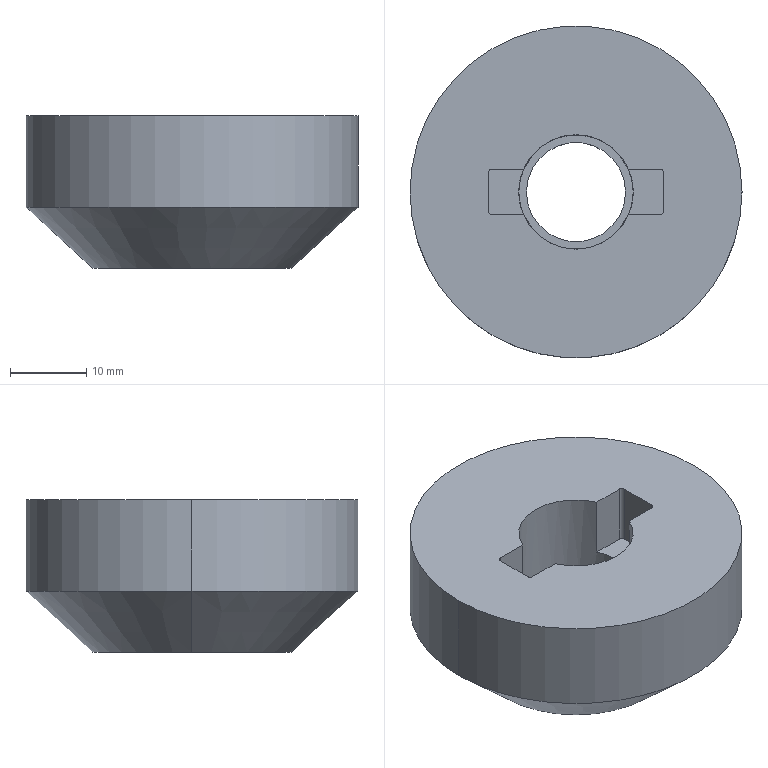Part | SolidWorks | features ICE 2, Blend 1, Extrusion 1 | 1 solid | 23 faces | box 43.5 x 43.5 x 20 mm | volume 21997 mm3 | plane 11 | cylinder 10 | cone 2 | commonest cylinder face diameters 1 x4 13 x2 15 x2 43.5 x2
STEP:
#1=CARTESIAN_POINT('',(6.5,0.,-8.));
#2=VERTEX_POINT('',#1);
#3=CARTESIAN_POINT('',(-6.5,0.,-8.));
#4=VERTEX_POINT('',#3);
#5=CARTESIAN_POINT('',(0.,0.,-8.));
#6=DIRECTION('',(0.,0.,-1.));
#7=DIRECTION('',(-1.,0.,0.));
#8=AXIS2_PLACEMENT_3D('',#5,#6,#7);
#9=CIRCLE('',#8,6.5);
#10=EDGE_CURVE('',#2,#4,#9,.T.);
#11=ORIENTED_EDGE('',*,*,#10,.T.);
#12=CARTESIAN_POINT('',(-6.5,0.,0.));
#13=VERTEX_POINT('',#12);
#14=CARTESIAN_POINT('',(-6.5,0.,-48.));
#15=DIRECTION('',(0.,0.,1.));
#16=VECTOR('',#15,1000.);
#17=LINE('',#14,#16);
#18=EDGE_CURVE('',#4,#13,#17,.T.);
#19=ORIENTED_EDGE('',*,*,#18,.T.);
#20=CARTESIAN_POINT('',(6.5,0.,0.));
#21=VERTEX_POINT('',#20);
#22=CARTESIAN_POINT('',(0.,0.,0.));
#23=DIRECTION('',(0.,0.,1.));
#24=DIRECTION('',(1.,0.,0.));
#25=AXIS2_PLACEMENT_3D('',#22,#23,#24);
#26=CIRCLE('',#25,6.5);
#27=EDGE_CURVE('',#13,#21,#26,.T.);
#28=ORIENTED_EDGE('',*,*,#27,.T.);
#29=CARTESIAN_POINT('',(6.5,0.,-48.));
#30=DIRECTION('',(0.,0.,1.));
#31=VECTOR('',#30,1000.);
#32=LINE('',#29,#31);
#33=EDGE_CURVE('',#2,#21,#32,.T.);
#34=ORIENTED_EDGE('',*,*,#33,.F.);
#35=EDGE_LOOP('',(#11,#19,#28,#34));
#36=FACE_OUTER_BOUND('',#35,.T.);
#37=CARTESIAN_POINT('',(0.,0.,-48.));
#38=DIRECTION('',(0.,0.,1.));
#39=DIRECTION('',(1.,0.,0.));
#40=AXIS2_PLACEMENT_3D('',#37,#38,#39);
#41=CYLINDRICAL_SURFACE('',#40,6.5);
#42=ADVANCED_FACE('',(#36),#41,.F.);
#43=CARTESIAN_POINT('',(-13.,0.,-8.));
#44=VERTEX_POINT('',#43);
#45=CARTESIAN_POINT('',(13.,0.,-8.));
#46=VERTEX_POINT('',#45);
#47=CARTESIAN_POINT('',(0.,0.,-8.));
#48=DIRECTION('',(0.,0.,-1.));
#49=DIRECTION('',(-1.,0.,0.));
#50=AXIS2_PLACEMENT_3D('',#47,#48,#49);
#51=CIRCLE('',#50,13.);
#52=EDGE_CURVE('',#44,#46,#51,.T.);
#53=ORIENTED_EDGE('',*,*,#52,.F.);
#54=CARTESIAN_POINT('',(-21.75,0.,0.));
#55=VERTEX_POINT('',#54);
#56=CARTESIAN_POINT('',(-13.,0.,-8.));
#57=DIRECTION('',(-0.738,0.,0.6748));
#58=VECTOR('',#57,1000.);
#59=LINE('',#56,#58);
#60=EDGE_CURVE('',#44,#55,#59,.T.);
#61=ORIENTED_EDGE('',*,*,#60,.T.);
#62=CARTESIAN_POINT('',(21.75,0.,0.));
#63=VERTEX_POINT('',#62);
#64=CARTESIAN_POINT('',(0.,0.,0.));
#65=DIRECTION('',(0.,0.,-1.));
#66=DIRECTION('',(-1.,0.,0.));
#67=AXIS2_PLACEMENT_3D('',#64,#65,#66);
#68=CIRCLE('',#67,21.75);
#69=EDGE_CURVE('',#55,#63,#68,.T.);
#70=ORIENTED_EDGE('',*,*,#69,.T.);
#71=CARTESIAN_POINT('',(13.,0.,-8.));
#72=DIRECTION('',(0.738,0.,0.6748));
#73=VECTOR('',#72,1000.);
#74=LINE('',#71,#73);
#75=EDGE_CURVE('',#46,#63,#74,.T.);
#76=ORIENTED_EDGE('',*,*,#75,.F.);
#77=EDGE_LOOP('',(#53,#61,#70,#76));
#78=FACE_OUTER_BOUND('',#77,.T.);
#79=CARTESIAN_POINT('',(0.,0.,-8.));
#80=DIRECTION('',(0.,0.,1.));
#81=DIRECTION('',(1.,0.,0.));
#82=AXIS2_PLACEMENT_3D('',#79,#80,#81);
#83=CONICAL_SURFACE('',#82,13.,0.8301);
#84=ADVANCED_FACE('',(#78),#83,.T.);
#85=CARTESIAN_POINT('',(7.5,0.,4.));
#86=VERTEX_POINT('',#85);
#87=CARTESIAN_POINT('',(6.874,-3.,4.));
#88=VERTEX_POINT('',#87);
#89=CARTESIAN_POINT('',(0.,0.,4.));
#90=DIRECTION('',(0.,0.,-1.));
#91=DIRECTION('',(-1.,0.,0.));
#92=AXIS2_PLACEMENT_3D('',#89,#90,#91);
#93=CIRCLE('',#92,7.5);
#94=EDGE_CURVE('',#86,#88,#93,.T.);
#95=ORIENTED_EDGE('',*,*,#94,.F.);
#96=CARTESIAN_POINT('',(7.5,0.,0.));
#97=VERTEX_POINT('',#96);
#98=CARTESIAN_POINT('',(7.5,0.,12.));
#99=DIRECTION('',(0.,0.,-1.));
#100=VECTOR('',#99,1000.);
#101=LINE('',#98,#100);
#102=EDGE_CURVE('',#86,#97,#101,.T.);
#103=ORIENTED_EDGE('',*,*,#102,.T.);
#104=CARTESIAN_POINT('',(-7.5,0.,0.));
#105=VERTEX_POINT('',#104);
#106=CARTESIAN_POINT('',(0.,0.,0.));
#107=DIRECTION('',(0.,0.,1.));
#108=DIRECTION('',(1.,0.,0.));
#109=AXIS2_PLACEMENT_3D('',#106,#107,#108);
#110=CIRCLE('',#109,7.5);
#111=EDGE_CURVE('',#105,#97,#110,.T.);
#112=ORIENTED_EDGE('',*,*,#111,.F.);
#113=CARTESIAN_POINT('',(-7.5,0.,4.));
#114=VERTEX_POINT('',#113);
#115=CARTESIAN_POINT('',(-7.5,0.,12.));
#116=DIRECTION('',(0.,0.,-1.));
#117=VECTOR('',#116,1000.);
#118=LINE('',#115,#117);
#119=EDGE_CURVE('',#114,#105,#118,.T.);
#120=ORIENTED_EDGE('',*,*,#119,.F.);
#121=CARTESIAN_POINT('',(-6.874,-3.,4.));
#122=VERTEX_POINT('',#121);
#123=CARTESIAN_POINT('',(0.,0.,4.));
#124=DIRECTION('',(0.,0.,-1.));
#125=DIRECTION('',(-1.,0.,0.));
#126=AXIS2_PLACEMENT_3D('',#123,#124,#125);
#127=CIRCLE('',#126,7.5);
#128=EDGE_CURVE('',#122,#114,#127,.T.);
#129=ORIENTED_EDGE('',*,*,#128,.F.);
#130=CARTESIAN_POINT('',(-6.874,-3.,12.));
#131=VERTEX_POINT('',#130);
#132=CARTESIAN_POINT('',(-6.874,-3.,12.));
#133=DIRECTION('',(0.,0.,-1.));
#134=VECTOR('',#133,1000.);
#135=LINE('',#132,#134);
#136=EDGE_CURVE('',#131,#122,#135,.T.);
#137=ORIENTED_EDGE('',*,*,#136,.F.);
#138=CARTESIAN_POINT('',(6.874,-3.,12.));
#139=VERTEX_POINT('',#138);
#140=CARTESIAN_POINT('',(0.,0.,12.));
#141=DIRECTION('',(0.,0.,1.));
#142=DIRECTION('',(1.,0.,0.));
#143=AXIS2_PLACEMENT_3D('',#140,#141,#142);
#144=CIRCLE('',#143,7.5);
#145=EDGE_CURVE('',#131,#139,#144,.T.);
#146=ORIENTED_EDGE('',*,*,#145,.T.);
#147=CARTESIAN_POINT('',(6.874,-3.,12.));
#148=DIRECTION('',(0.,0.,1.));
#149=VECTOR('',#148,1000.);
#150=LINE('',#147,#149);
#151=EDGE_CURVE('',#88,#139,#150,.T.);
#152=ORIENTED_EDGE('',*,*,#151,.F.);
#153=EDGE_LOOP('',(#95,#103,#112,#120,#129,#137,#146,#152));
#154=FACE_OUTER_BOUND('',#153,.T.);
#155=CARTESIAN_POINT('',(0.,0.,12.));
#156=DIRECTION('',(0.,0.,-1.));
#157=DIRECTION('',(-1.,0.,0.));
#158=AXIS2_PLACEMENT_3D('',#155,#156,#157);
#159=CYLINDRICAL_SURFACE('',#158,7.5);
#160=ADVANCED_FACE('',(#154),#159,.F.);
#161=CARTESIAN_POINT('',(21.75,0.,12.));
#162=VERTEX_POINT('',#161);
#163=CARTESIAN_POINT('',(-21.75,0.,12.));
#164=VERTEX_POINT('',#163);
#165=CARTESIAN_POINT('',(0.,0.,12.));
#166=DIRECTION('',(0.,0.,1.));
#167=DIRECTION('',(1.,0.,0.));
#168=AXIS2_PLACEMENT_3D('',#165,#166,#167);
#169=CIRCLE('',#168,21.75);
#170=EDGE_CURVE('',#162,#164,#169,.T.);
#171=ORIENTED_EDGE('',*,*,#170,.F.);
#172=CARTESIAN_POINT('',(21.75,0.,12.));
#173=DIRECTION('',(0.,0.,-1.));
#174=VECTOR('',#173,1000.);
#175=LINE('',#172,#174);
#176=EDGE_CURVE('',#162,#63,#175,.T.);
#177=ORIENTED_EDGE('',*,*,#176,.T.);
#178=ORIENTED_EDGE('',*,*,#69,.F.);
#179=CARTESIAN_POINT('',(-21.75,0.,12.));
#180=DIRECTION('',(0.,0.,-1.));
#181=VECTOR('',#180,1000.);
#182=LINE('',#179,#181);
#183=EDGE_CURVE('',#164,#55,#182,.T.);
#184=ORIENTED_EDGE('',*,*,#183,.F.);
#185=EDGE_LOOP('',(#171,#177,#178,#184));
#186=FACE_OUTER_BOUND('',#185,.T.);
#187=CARTESIAN_POINT('',(0.,0.,12.));
#188=DIRECTION('',(0.,0.,-1.));
#189=DIRECTION('',(-1.,0.,0.));
#190=AXIS2_PLACEMENT_3D('',#187,#188,#189);
#191=CYLINDRICAL_SURFACE('',#190,21.75);
#192=ADVANCED_FACE('',(#186),#191,.T.);
#193=CARTESIAN_POINT('',(11.,-3.,12.));
#194=VERTEX_POINT('',#193);
#195=CARTESIAN_POINT('',(-11.,-3.,12.));
#196=DIRECTION('',(1.,0.,0.));
#197=VECTOR('',#196,1000.);
#198=LINE('',#195,#197);
#199=EDGE_CURVE('',#139,#194,#198,.T.);
#200=ORIENTED_EDGE('',*,*,#199,.F.);
#201=ORIENTED_EDGE('',*,*,#145,.F.);
#202=CARTESIAN_POINT('',(-11.,-3.,12.));
#203=VERTEX_POINT('',#202);
#204=CARTESIAN_POINT('',(-11.,-3.,12.));
#205=DIRECTION('',(1.,0.,0.));
#206=VECTOR('',#205,1000.);
#207=LINE('',#204,#206);
#208=EDGE_CURVE('',#203,#131,#207,.T.);
#209=ORIENTED_EDGE('',*,*,#208,.F.);
#210=CARTESIAN_POINT('',(-11.5,-2.5,12.));
#211=VERTEX_POINT('',#210);
#212=CARTESIAN_POINT('',(-11.,-2.5,12.));
#213=DIRECTION('',(0.,0.,1.));
#214=DIRECTION('',(1.,0.,0.));
#215=AXIS2_PLACEMENT_3D('',#212,#213,#214);
#216=CIRCLE('',#215,0.5);
#217=EDGE_CURVE('',#211,#203,#216,.T.);
#218=ORIENTED_EDGE('',*,*,#217,.F.);
#219=CARTESIAN_POINT('',(-11.5,2.5,12.));
#220=VERTEX_POINT('',#219);
#221=CARTESIAN_POINT('',(-11.5,2.5,12.));
#222=DIRECTION('',(0.,-1.,0.));
#223=VECTOR('',#222,1000.);
#224=LINE('',#221,#223);
#225=EDGE_CURVE('',#220,#211,#224,.T.);
#226=ORIENTED_EDGE('',*,*,#225,.F.);
#227=CARTESIAN_POINT('',(-11.,3.,12.));
#228=VERTEX_POINT('',#227);
#229=CARTESIAN_POINT('',(-11.,2.5,12.));
#230=DIRECTION('',(0.,0.,1.));
#231=DIRECTION('',(1.,0.,0.));
#232=AXIS2_PLACEMENT_3D('',#229,#230,#231);
#233=CIRCLE('',#232,0.5);
#234=EDGE_CURVE('',#228,#220,#233,.T.);
#235=ORIENTED_EDGE('',*,*,#234,.F.);
#236=CARTESIAN_POINT('',(-6.874,3.,12.));
#237=VERTEX_POINT('',#236);
#238=CARTESIAN_POINT('',(-11.,3.,12.));
#239=DIRECTION('',(-1.,0.,0.));
#240=VECTOR('',#239,1000.);
#241=LINE('',#238,#240);
#242=EDGE_CURVE('',#237,#228,#241,.T.);
#243=ORIENTED_EDGE('',*,*,#242,.F.);
#244=CARTESIAN_POINT('',(6.874,3.,12.));
#245=VERTEX_POINT('',#244);
#246=CARTESIAN_POINT('',(0.,0.,12.));
#247=DIRECTION('',(0.,0.,1.));
#248=DIRECTION('',(1.,0.,0.));
#249=AXIS2_PLACEMENT_3D('',#246,#247,#248);
#250=CIRCLE('',#249,7.5);
#251=EDGE_CURVE('',#245,#237,#250,.T.);
#252=ORIENTED_EDGE('',*,*,#251,.F.);
#253=CARTESIAN_POINT('',(11.,3.,12.));
#254=VERTEX_POINT('',#253);
#255=CARTESIAN_POINT('',(-11.,3.,12.));
#256=DIRECTION('',(-1.,0.,0.));
#257=VECTOR('',#256,1000.);
#258=LINE('',#255,#257);
#259=EDGE_CURVE('',#254,#245,#258,.T.);
#260=ORIENTED_EDGE('',*,*,#259,.F.);
#261=CARTESIAN_POINT('',(11.5,2.5,12.));
#262=VERTEX_POINT('',#261);
#263=CARTESIAN_POINT('',(11.,2.5,12.));
#264=DIRECTION('',(0.,0.,1.));
#265=DIRECTION('',(-1.,0.,0.));
#266=AXIS2_PLACEMENT_3D('',#263,#264,#265);
#267=CIRCLE('',#266,0.5);
#268=EDGE_CURVE('',#262,#254,#267,.T.);
#269=ORIENTED_EDGE('',*,*,#268,.F.);
#270=CARTESIAN_POINT('',(11.5,-2.5,12.));
#271=VERTEX_POINT('',#270);
#272=CARTESIAN_POINT('',(11.5,2.5,12.));
#273=DIRECTION('',(0.,1.,0.));
#274=VECTOR('',#273,1000.);
#275=LINE('',#272,#274);
#276=EDGE_CURVE('',#271,#262,#275,.T.);
#277=ORIENTED_EDGE('',*,*,#276,.F.);
#278=CARTESIAN_POINT('',(11.,-2.5,12.));
#279=DIRECTION('',(0.,0.,1.));
#280=DIRECTION('',(1.,0.,0.));
#281=AXIS2_PLACEMENT_3D('',#278,#279,#280);
#282=CIRCLE('',#281,0.5);
#283=EDGE_CURVE('',#194,#271,#282,.T.);
#284=ORIENTED_EDGE('',*,*,#283,.F.);
#285=EDGE_LOOP('',(#200,#201,#209,#218,#226,#235,#243,#252,#260,#269,#277,#284));
#286=FACE_BOUND('',#285,.T.);
#287=CARTESIAN_POINT('',(0.,0.,12.));
#288=DIRECTION('',(0.,0.,1.));
#289=DIRECTION('',(1.,0.,0.));
#290=AXIS2_PLACEMENT_3D('',#287,#288,#289);
#291=CIRCLE('',#290,21.75);
#292=EDGE_CURVE('',#164,#162,#291,.T.);
#293=ORIENTED_EDGE('',*,*,#292,.T.);
#294=ORIENTED_EDGE('',*,*,#170,.T.);
#295=EDGE_LOOP('',(#293,#294));
#296=FACE_OUTER_BOUND('',#295,.T.);
#297=CARTESIAN_POINT('',(0.,0.,12.));
#298=DIRECTION('',(0.,0.,1.));
#299=DIRECTION('',(1.,0.,0.));
#300=AXIS2_PLACEMENT_3D('',#297,#298,#299);
#301=PLANE('',#300);
#302=ADVANCED_FACE('',(#286,#296),#301,.T.);
#303=ORIENTED_EDGE('',*,*,#176,.F.);
#304=ORIENTED_EDGE('',*,*,#292,.F.);
#305=ORIENTED_EDGE('',*,*,#183,.T.);
#306=CARTESIAN_POINT('',(0.,0.,0.));
#307=DIRECTION('',(0.,0.,-1.));
#308=DIRECTION('',(-1.,0.,0.));
#309=AXIS2_PLACEMENT_3D('',#306,#307,#308);
#310=CIRCLE('',#309,21.75);
#311=EDGE_CURVE('',#63,#55,#310,.T.);
#312=ORIENTED_EDGE('',*,*,#311,.F.);
#313=EDGE_LOOP('',(#303,#304,#305,#312));
#314=FACE_OUTER_BOUND('',#313,.T.);
#315=CARTESIAN_POINT('',(0.,0.,12.));
#316=DIRECTION('',(0.,0.,-1.));
#317=DIRECTION('',(-1.,0.,0.));
#318=AXIS2_PLACEMENT_3D('',#315,#316,#317);
#319=CYLINDRICAL_SURFACE('',#318,21.75);
#320=ADVANCED_FACE('',(#314),#319,.T.);
#321=ORIENTED_EDGE('',*,*,#102,.F.);
#322=CARTESIAN_POINT('',(6.874,3.,4.));
#323=VERTEX_POINT('',#322);
#324=CARTESIAN_POINT('',(0.,0.,4.));
#325=DIRECTION('',(0.,0.,-1.));
#326=DIRECTION('',(-1.,0.,0.));
#327=AXIS2_PLACEMENT_3D('',#324,#325,#326);
#328=CIRCLE('',#327,7.5);
#329=EDGE_CURVE('',#323,#86,#328,.T.);
#330=ORIENTED_EDGE('',*,*,#329,.F.);
#331=CARTESIAN_POINT('',(6.874,3.,12.));
#332=DIRECTION('',(0.,0.,-1.));
#333=VECTOR('',#332,1000.);
#334=LINE('',#331,#333);
#335=EDGE_CURVE('',#245,#323,#334,.T.);
#336=ORIENTED_EDGE('',*,*,#335,.F.);
#337=ORIENTED_EDGE('',*,*,#251,.T.);
#338=CARTESIAN_POINT('',(-6.874,3.,4.));
#339=VERTEX_POINT('',#338);
#340=CARTESIAN_POINT('',(-6.874,3.,12.));
#341=DIRECTION('',(0.,0.,1.));
#342=VECTOR('',#341,1000.);
#343=LINE('',#340,#342);
#344=EDGE_CURVE('',#339,#237,#343,.T.);
#345=ORIENTED_EDGE('',*,*,#344,.F.);
#346=CARTESIAN_POINT('',(0.,0.,4.));
#347=DIRECTION('',(0.,0.,-1.));
#348=DIRECTION('',(-1.,0.,0.));
#349=AXIS2_PLACEMENT_3D('',#346,#347,#348);
#350=CIRCLE('',#349,7.5);
#351=EDGE_CURVE('',#114,#339,#350,.T.);
#352=ORIENTED_EDGE('',*,*,#351,.F.);
#353=ORIENTED_EDGE('',*,*,#119,.T.);
#354=CARTESIAN_POINT('',(0.,0.,0.));
#355=DIRECTION('',(0.,0.,1.));
#356=DIRECTION('',(1.,0.,0.));
#357=AXIS2_PLACEMENT_3D('',#354,#355,#356);
#358=CIRCLE('',#357,7.5);
#359=EDGE_CURVE('',#97,#105,#358,.T.);
#360=ORIENTED_EDGE('',*,*,#359,.F.);
#361=EDGE_LOOP('',(#321,#330,#336,#337,#345,#352,#353,#360));
#362=FACE_OUTER_BOUND('',#361,.T.);
#363=CARTESIAN_POINT('',(0.,0.,12.));
#364=DIRECTION('',(0.,0.,-1.));
#365=DIRECTION('',(-1.,0.,0.));
#366=AXIS2_PLACEMENT_3D('',#363,#364,#365);
#367=CYLINDRICAL_SURFACE('',#366,7.5);
#368=ADVANCED_FACE('',(#362),#367,.F.);
#369=ORIENTED_EDGE('',*,*,#128,.T.);
#370=ORIENTED_EDGE('',*,*,#351,.T.);
#371=CARTESIAN_POINT('',(-11.,3.,4.));
#372=VERTEX_POINT('',#371);
#373=CARTESIAN_POINT('',(-11.,3.,4.));
#374=DIRECTION('',(-1.,0.,0.));
#375=VECTOR('',#374,1000.);
#376=LINE('',#373,#375);
#377=EDGE_CURVE('',#339,#372,#376,.T.);
#378=ORIENTED_EDGE('',*,*,#377,.T.);
#379=CARTESIAN_POINT('',(-11.5,2.5,4.));
#380=VERTEX_POINT('',#379);
#381=CARTESIAN_POINT('',(-11.,2.5,4.));
#382=DIRECTION('',(0.,0.,1.));
#383=DIRECTION('',(1.,0.,0.));
#384=AXIS2_PLACEMENT_3D('',#381,#382,#383);
#385=CIRCLE('',#384,0.5);
#386=EDGE_CURVE('',#372,#380,#385,.T.);
#387=ORIENTED_EDGE('',*,*,#386,.T.);
#388=CARTESIAN_POINT('',(-11.5,-2.5,4.));
#389=VERTEX_POINT('',#388);
#390=CARTESIAN_POINT('',(-11.5,2.5,4.));
#391=DIRECTION('',(0.,-1.,0.));
#392=VECTOR('',#391,1000.);
#393=LINE('',#390,#392);
#394=EDGE_CURVE('',#380,#389,#393,.T.);
#395=ORIENTED_EDGE('',*,*,#394,.T.);
#396=CARTESIAN_POINT('',(-11.,-3.,4.));
#397=VERTEX_POINT('',#396);
#398=CARTESIAN_POINT('',(-11.,-2.5,4.));
#399=DIRECTION('',(0.,0.,1.));
#400=DIRECTION('',(1.,0.,0.));
#401=AXIS2_PLACEMENT_3D('',#398,#399,#400);
#402=CIRCLE('',#401,0.5);
#403=EDGE_CURVE('',#389,#397,#402,.T.);
#404=ORIENTED_EDGE('',*,*,#403,.T.);
#405=CARTESIAN_POINT('',(-11.,-3.,4.));
#406=DIRECTION('',(1.,0.,0.));
#407=VECTOR('',#406,1000.);
#408=LINE('',#405,#407);
#409=EDGE_CURVE('',#397,#122,#408,.T.);
#410=ORIENTED_EDGE('',*,*,#409,.T.);
#411=EDGE_LOOP('',(#369,#370,#378,#387,#395,#404,#410));
#412=FACE_OUTER_BOUND('',#411,.T.);
#413=CARTESIAN_POINT('',(11.,2.5,4.));
#414=DIRECTION('',(0.,0.,-1.));
#415=DIRECTION('',(-1.,0.,0.));
#416=AXIS2_PLACEMENT_3D('',#413,#414,#415);
#417=PLANE('',#416);
#418=ADVANCED_FACE('',(#412),#417,.F.);
#419=ORIENTED_EDGE('',*,*,#344,.T.);
#420=ORIENTED_EDGE('',*,*,#242,.T.);
#421=CARTESIAN_POINT('',(-11.,3.,4.));
#422=DIRECTION('',(0.,0.,1.));
#423=VECTOR('',#422,1000.);
#424=LINE('',#421,#423);
#425=EDGE_CURVE('',#372,#228,#424,.T.);
#426=ORIENTED_EDGE('',*,*,#425,.F.);
#427=ORIENTED_EDGE('',*,*,#377,.F.);
#428=EDGE_LOOP('',(#419,#420,#426,#427));
#429=FACE_OUTER_BOUND('',#428,.T.);
#430=CARTESIAN_POINT('',(-11.,3.,4.));
#431=DIRECTION('',(0.,1.,0.));
#432=DIRECTION('',(0.,0.,1.));
#433=AXIS2_PLACEMENT_3D('',#430,#431,#432);
#434=PLANE('',#433);
#435=ADVANCED_FACE('',(#429),#434,.F.);
#436=ORIENTED_EDGE('',*,*,#136,.T.);
#437=ORIENTED_EDGE('',*,*,#409,.F.);
#438=CARTESIAN_POINT('',(-11.,-3.,4.));
#439=DIRECTION('',(0.,0.,1.));
#440=VECTOR('',#439,1000.);
#441=LINE('',#438,#440);
#442=EDGE_CURVE('',#397,#203,#441,.T.);
#443=ORIENTED_EDGE('',*,*,#442,.T.);
#444=ORIENTED_EDGE('',*,*,#208,.T.);
#445=EDGE_LOOP('',(#436,#437,#443,#444));
#446=FACE_OUTER_BOUND('',#445,.T.);
#447=CARTESIAN_POINT('',(-11.,-3.,4.));
#448=DIRECTION('',(0.,-1.,0.));
#449=DIRECTION('',(0.,0.,-1.));
#450=AXIS2_PLACEMENT_3D('',#447,#448,#449);
#451=PLANE('',#450);
#452=ADVANCED_FACE('',(#446),#451,.F.);
#453=ORIENTED_EDGE('',*,*,#234,.T.);
#454=CARTESIAN_POINT('',(-11.5,2.5,4.));
#455=DIRECTION('',(0.,0.,1.));
#456=VECTOR('',#455,1000.);
#457=LINE('',#454,#456);
#458=EDGE_CURVE('',#380,#220,#457,.T.);
#459=ORIENTED_EDGE('',*,*,#458,.F.);
#460=ORIENTED_EDGE('',*,*,#386,.F.);
#461=ORIENTED_EDGE('',*,*,#425,.T.);
#462=EDGE_LOOP('',(#453,#459,#460,#461));
#463=FACE_OUTER_BOUND('',#462,.T.);
#464=CARTESIAN_POINT('',(-11.,2.5,4.));
#465=DIRECTION('',(0.,0.,1.));
#466=DIRECTION('',(1.,0.,0.));
#467=AXIS2_PLACEMENT_3D('',#464,#465,#466);
#468=CYLINDRICAL_SURFACE('',#467,0.5);
#469=ADVANCED_FACE('',(#463),#468,.F.);
#470=ORIENTED_EDGE('',*,*,#225,.T.);
#471=CARTESIAN_POINT('',(-11.5,-2.5,4.));
#472=DIRECTION('',(0.,0.,1.));
#473=VECTOR('',#472,1000.);
#474=LINE('',#471,#473);
#475=EDGE_CURVE('',#389,#211,#474,.T.);
#476=ORIENTED_EDGE('',*,*,#475,.F.);
#477=ORIENTED_EDGE('',*,*,#394,.F.);
#478=ORIENTED_EDGE('',*,*,#458,.T.);
#479=EDGE_LOOP('',(#470,#476,#477,#478));
#480=FACE_OUTER_BOUND('',#479,.T.);
#481=CARTESIAN_POINT('',(-11.5,2.5,4.));
#482=DIRECTION('',(-1.,0.,0.));
#483=DIRECTION('',(0.,0.,1.));
#484=AXIS2_PLACEMENT_3D('',#481,#482,#483);
#485=PLANE('',#484);
#486=ADVANCED_FACE('',(#480),#485,.F.);
#487=ORIENTED_EDGE('',*,*,#217,.T.);
#488=ORIENTED_EDGE('',*,*,#442,.F.);
#489=ORIENTED_EDGE('',*,*,#403,.F.);
#490=ORIENTED_EDGE('',*,*,#475,.T.);
#491=EDGE_LOOP('',(#487,#488,#489,#490));
#492=FACE_OUTER_BOUND('',#491,.T.);
#493=CARTESIAN_POINT('',(-11.,-2.5,4.));
#494=DIRECTION('',(0.,0.,1.));
#495=DIRECTION('',(1.,0.,0.));
#496=AXIS2_PLACEMENT_3D('',#493,#494,#495);
#497=CYLINDRICAL_SURFACE('',#496,0.5);
#498=ADVANCED_FACE('',(#492),#497,.F.);
#499=ORIENTED_EDGE('',*,*,#335,.T.);
#500=CARTESIAN_POINT('',(11.,3.,4.));
#501=VERTEX_POINT('',#500);
#502=CARTESIAN_POINT('',(-11.,3.,4.));
#503=DIRECTION('',(-1.,0.,0.));
#504=VECTOR('',#503,1000.);
#505=LINE('',#502,#504);
#506=EDGE_CURVE('',#501,#323,#505,.T.);
#507=ORIENTED_EDGE('',*,*,#506,.F.);
#508=CARTESIAN_POINT('',(11.,3.,4.));
#509=DIRECTION('',(0.,0.,1.));
#510=VECTOR('',#509,1000.);
#511=LINE('',#508,#510);
#512=EDGE_CURVE('',#501,#254,#511,.T.);
#513=ORIENTED_EDGE('',*,*,#512,.T.);
#514=ORIENTED_EDGE('',*,*,#259,.T.);
#515=EDGE_LOOP('',(#499,#507,#513,#514));
#516=FACE_OUTER_BOUND('',#515,.T.);
#517=CARTESIAN_POINT('',(-11.,3.,4.));
#518=DIRECTION('',(0.,1.,0.));
#519=DIRECTION('',(0.,0.,1.));
#520=AXIS2_PLACEMENT_3D('',#517,#518,#519);
#521=PLANE('',#520);
#522=ADVANCED_FACE('',(#516),#521,.F.);
#523=ORIENTED_EDGE('',*,*,#329,.T.);
#524=ORIENTED_EDGE('',*,*,#94,.T.);
#525=CARTESIAN_POINT('',(11.,-3.,4.));
#526=VERTEX_POINT('',#525);
#527=CARTESIAN_POINT('',(-11.,-3.,4.));
#528=DIRECTION('',(1.,0.,0.));
#529=VECTOR('',#528,1000.);
#530=LINE('',#527,#529);
#531=EDGE_CURVE('',#88,#526,#530,.T.);
#532=ORIENTED_EDGE('',*,*,#531,.T.);
#533=CARTESIAN_POINT('',(11.5,-2.5,4.));
#534=VERTEX_POINT('',#533);
#535=CARTESIAN_POINT('',(11.,-2.5,4.));
#536=DIRECTION('',(0.,0.,1.));
#537=DIRECTION('',(1.,0.,0.));
#538=AXIS2_PLACEMENT_3D('',#535,#536,#537);
#539=CIRCLE('',#538,0.5);
#540=EDGE_CURVE('',#526,#534,#539,.T.);
#541=ORIENTED_EDGE('',*,*,#540,.T.);
#542=CARTESIAN_POINT('',(11.5,2.5,4.));
#543=VERTEX_POINT('',#542);
#544=CARTESIAN_POINT('',(11.5,2.5,4.));
#545=DIRECTION('',(0.,1.,0.));
#546=VECTOR('',#545,1000.);
#547=LINE('',#544,#546);
#548=EDGE_CURVE('',#534,#543,#547,.T.);
#549=ORIENTED_EDGE('',*,*,#548,.T.);
#550=CARTESIAN_POINT('',(11.,2.5,4.));
#551=DIRECTION('',(0.,0.,1.));
#552=DIRECTION('',(-1.,0.,0.));
#553=AXIS2_PLACEMENT_3D('',#550,#551,#552);
#554=CIRCLE('',#553,0.5);
#555=EDGE_CURVE('',#543,#501,#554,.T.);
#556=ORIENTED_EDGE('',*,*,#555,.T.);
#557=ORIENTED_EDGE('',*,*,#506,.T.);
#558=EDGE_LOOP('',(#523,#524,#532,#541,#549,#556,#557));
#559=FACE_OUTER_BOUND('',#558,.T.);
#560=CARTESIAN_POINT('',(11.,2.5,4.));
#561=DIRECTION('',(0.,0.,-1.));
#562=DIRECTION('',(-1.,0.,0.));
#563=AXIS2_PLACEMENT_3D('',#560,#561,#562);
#564=PLANE('',#563);
#565=ADVANCED_FACE('',(#559),#564,.F.);
#566=ORIENTED_EDGE('',*,*,#268,.T.);
#567=ORIENTED_EDGE('',*,*,#512,.F.);
#568=ORIENTED_EDGE('',*,*,#555,.F.);
#569=CARTESIAN_POINT('',(11.5,2.5,4.));
#570=DIRECTION('',(0.,0.,1.));
#571=VECTOR('',#570,1000.);
#572=LINE('',#569,#571);
#573=EDGE_CURVE('',#543,#262,#572,.T.);
#574=ORIENTED_EDGE('',*,*,#573,.T.);
#575=EDGE_LOOP('',(#566,#567,#568,#574));
#576=FACE_OUTER_BOUND('',#575,.T.);
#577=CARTESIAN_POINT('',(11.,2.5,4.));
#578=DIRECTION('',(0.,0.,1.));
#579=DIRECTION('',(1.,0.,0.));
#580=AXIS2_PLACEMENT_3D('',#577,#578,#579);
#581=CYLINDRICAL_SURFACE('',#580,0.5);
#582=ADVANCED_FACE('',(#576),#581,.F.);
#583=ORIENTED_EDGE('',*,*,#276,.T.);
#584=ORIENTED_EDGE('',*,*,#573,.F.);
#585=ORIENTED_EDGE('',*,*,#548,.F.);
#586=CARTESIAN_POINT('',(11.5,-2.5,4.));
#587=DIRECTION('',(0.,0.,1.));
#588=VECTOR('',#587,1000.);
#589=LINE('',#586,#588);
#590=EDGE_CURVE('',#534,#271,#589,.T.);
#591=ORIENTED_EDGE('',*,*,#590,.T.);
#592=EDGE_LOOP('',(#583,#584,#585,#591));
#593=FACE_OUTER_BOUND('',#592,.T.);
#594=CARTESIAN_POINT('',(11.5,2.5,4.));
#595=DIRECTION('',(1.,0.,0.));
#596=DIRECTION('',(0.,1.,0.));
#597=AXIS2_PLACEMENT_3D('',#594,#595,#596);
#598=PLANE('',#597);
#599=ADVANCED_FACE('',(#593),#598,.F.);
#600=ORIENTED_EDGE('',*,*,#283,.T.);
#601=ORIENTED_EDGE('',*,*,#590,.F.);
#602=ORIENTED_EDGE('',*,*,#540,.F.);
#603=CARTESIAN_POINT('',(11.,-3.,4.));
#604=DIRECTION('',(0.,0.,1.));
#605=VECTOR('',#604,1000.);
#606=LINE('',#603,#605);
#607=EDGE_CURVE('',#526,#194,#606,.T.);
#608=ORIENTED_EDGE('',*,*,#607,.T.);
#609=EDGE_LOOP('',(#600,#601,#602,#608));
#610=FACE_OUTER_BOUND('',#609,.T.);
#611=CARTESIAN_POINT('',(11.,-2.5,4.));
#612=DIRECTION('',(0.,0.,1.));
#613=DIRECTION('',(1.,0.,0.));
#614=AXIS2_PLACEMENT_3D('',#611,#612,#613);
#615=CYLINDRICAL_SURFACE('',#614,0.5);
#616=ADVANCED_FACE('',(#610),#615,.F.);
#617=ORIENTED_EDGE('',*,*,#151,.T.);
#618=ORIENTED_EDGE('',*,*,#199,.T.);
#619=ORIENTED_EDGE('',*,*,#607,.F.);
#620=ORIENTED_EDGE('',*,*,#531,.F.);
#621=EDGE_LOOP('',(#617,#618,#619,#620));
#622=FACE_OUTER_BOUND('',#621,.T.);
#623=CARTESIAN_POINT('',(-11.,-3.,4.));
#624=DIRECTION('',(0.,-1.,0.));
#625=DIRECTION('',(0.,0.,-1.));
#626=AXIS2_PLACEMENT_3D('',#623,#624,#625);
#627=PLANE('',#626);
#628=ADVANCED_FACE('',(#622),#627,.F.);
#629=CARTESIAN_POINT('',(0.,0.,0.));
#630=DIRECTION('',(0.,0.,1.));
#631=DIRECTION('',(1.,0.,0.));
#632=AXIS2_PLACEMENT_3D('',#629,#630,#631);
#633=CIRCLE('',#632,6.5);
#634=EDGE_CURVE('',#21,#13,#633,.T.);
#635=ORIENTED_EDGE('',*,*,#634,.F.);
#636=ORIENTED_EDGE('',*,*,#27,.F.);
#637=EDGE_LOOP('',(#635,#636));
#638=FACE_BOUND('',#637,.T.);
#639=ORIENTED_EDGE('',*,*,#111,.T.);
#640=ORIENTED_EDGE('',*,*,#359,.T.);
#641=EDGE_LOOP('',(#639,#640));
#642=FACE_OUTER_BOUND('',#641,.T.);
#643=CARTESIAN_POINT('',(0.,0.,0.));
#644=DIRECTION('',(0.,0.,-1.));
#645=DIRECTION('',(-1.,0.,0.));
#646=AXIS2_PLACEMENT_3D('',#643,#644,#645);
#647=PLANE('',#646);
#648=ADVANCED_FACE('',(#638,#642),#647,.F.);
#649=ORIENTED_EDGE('',*,*,#10,.F.);
#650=CARTESIAN_POINT('',(0.,0.,-8.));
#651=DIRECTION('',(0.,0.,-1.));
#652=DIRECTION('',(-1.,0.,0.));
#653=AXIS2_PLACEMENT_3D('',#650,#651,#652);
#654=CIRCLE('',#653,6.5);
#655=EDGE_CURVE('',#4,#2,#654,.T.);
#656=ORIENTED_EDGE('',*,*,#655,.F.);
#657=EDGE_LOOP('',(#649,#656));
#658=FACE_BOUND('',#657,.T.);
#659=CARTESIAN_POINT('',(0.,0.,-8.));
#660=DIRECTION('',(0.,0.,-1.));
#661=DIRECTION('',(-1.,0.,0.));
#662=AXIS2_PLACEMENT_3D('',#659,#660,#661);
#663=CIRCLE('',#662,13.);
#664=EDGE_CURVE('',#46,#44,#663,.T.);
#665=ORIENTED_EDGE('',*,*,#664,.T.);
#666=ORIENTED_EDGE('',*,*,#52,.T.);
#667=EDGE_LOOP('',(#665,#666));
#668=FACE_OUTER_BOUND('',#667,.T.);
#669=CARTESIAN_POINT('',(0.,0.,-8.));
#670=DIRECTION('',(0.,0.,-1.));
#671=DIRECTION('',(-1.,0.,0.));
#672=AXIS2_PLACEMENT_3D('',#669,#670,#671);
#673=PLANE('',#672);
#674=ADVANCED_FACE('',(#658,#668),#673,.T.);
#675=ORIENTED_EDGE('',*,*,#60,.F.);
#676=ORIENTED_EDGE('',*,*,#664,.F.);
#677=ORIENTED_EDGE('',*,*,#75,.T.);
#678=ORIENTED_EDGE('',*,*,#311,.T.);
#679=EDGE_LOOP('',(#675,#676,#677,#678));
#680=FACE_OUTER_BOUND('',#679,.T.);
#681=CARTESIAN_POINT('',(0.,0.,-8.));
#682=DIRECTION('',(0.,0.,1.));
#683=DIRECTION('',(1.,0.,0.));
#684=AXIS2_PLACEMENT_3D('',#681,#682,#683);
#685=CONICAL_SURFACE('',#684,13.,0.8301);
#686=ADVANCED_FACE('',(#680),#685,.T.);
#687=ORIENTED_EDGE('',*,*,#18,.F.);
#688=ORIENTED_EDGE('',*,*,#655,.T.);
#689=ORIENTED_EDGE('',*,*,#33,.T.);
#690=ORIENTED_EDGE('',*,*,#634,.T.);
#691=EDGE_LOOP('',(#687,#688,#689,#690));
#692=FACE_OUTER_BOUND('',#691,.T.);
#693=CARTESIAN_POINT('',(0.,0.,-48.));
#694=DIRECTION('',(0.,0.,1.));
#695=DIRECTION('',(1.,0.,0.));
#696=AXIS2_PLACEMENT_3D('',#693,#694,#695);
#697=CYLINDRICAL_SURFACE('',#696,6.5);
#698=ADVANCED_FACE('',(#692),#697,.F.);
#699=CLOSED_SHELL('',(#42,#84,#160,#192,#302,#320,#368,#418,#435,#452,#469,#486,#498,#522,#565,#582,#599,#616,#628,#648,#674,#686,#698));
#700=MANIFOLD_SOLID_BREP('',#699);
#701=CARTESIAN_POINT('',(0.,0.,0.));
#702=DIRECTION('',(0.,0.,1.));
#703=DIRECTION('',(1.,0.,0.));
#704=AXIS2_PLACEMENT_3D('',#701,#702,#703);
#705=(LENGTH_UNIT()NAMED_UNIT(*)SI_UNIT(.MILLI.,.METRE.));
#706=UNCERTAINTY_MEASURE_WITH_UNIT(LENGTH_MEASURE(0.00001),#705,'','');
#707=(NAMED_UNIT(*)PLANE_ANGLE_UNIT()SI_UNIT($,.RADIAN.));
#708=(NAMED_UNIT(*)SI_UNIT($,.STERADIAN.)SOLID_ANGLE_UNIT());
#709=(GEOMETRIC_REPRESENTATION_CONTEXT(3)GLOBAL_UNCERTAINTY_ASSIGNED_CONTEXT((#706))GLOBAL_UNIT_ASSIGNED_CONTEXT((#705,#707,#708))REPRESENTATION_CONTEXT('',''));
#710=ADVANCED_BREP_SHAPE_REPRESENTATION('',(#700,#704),#709);